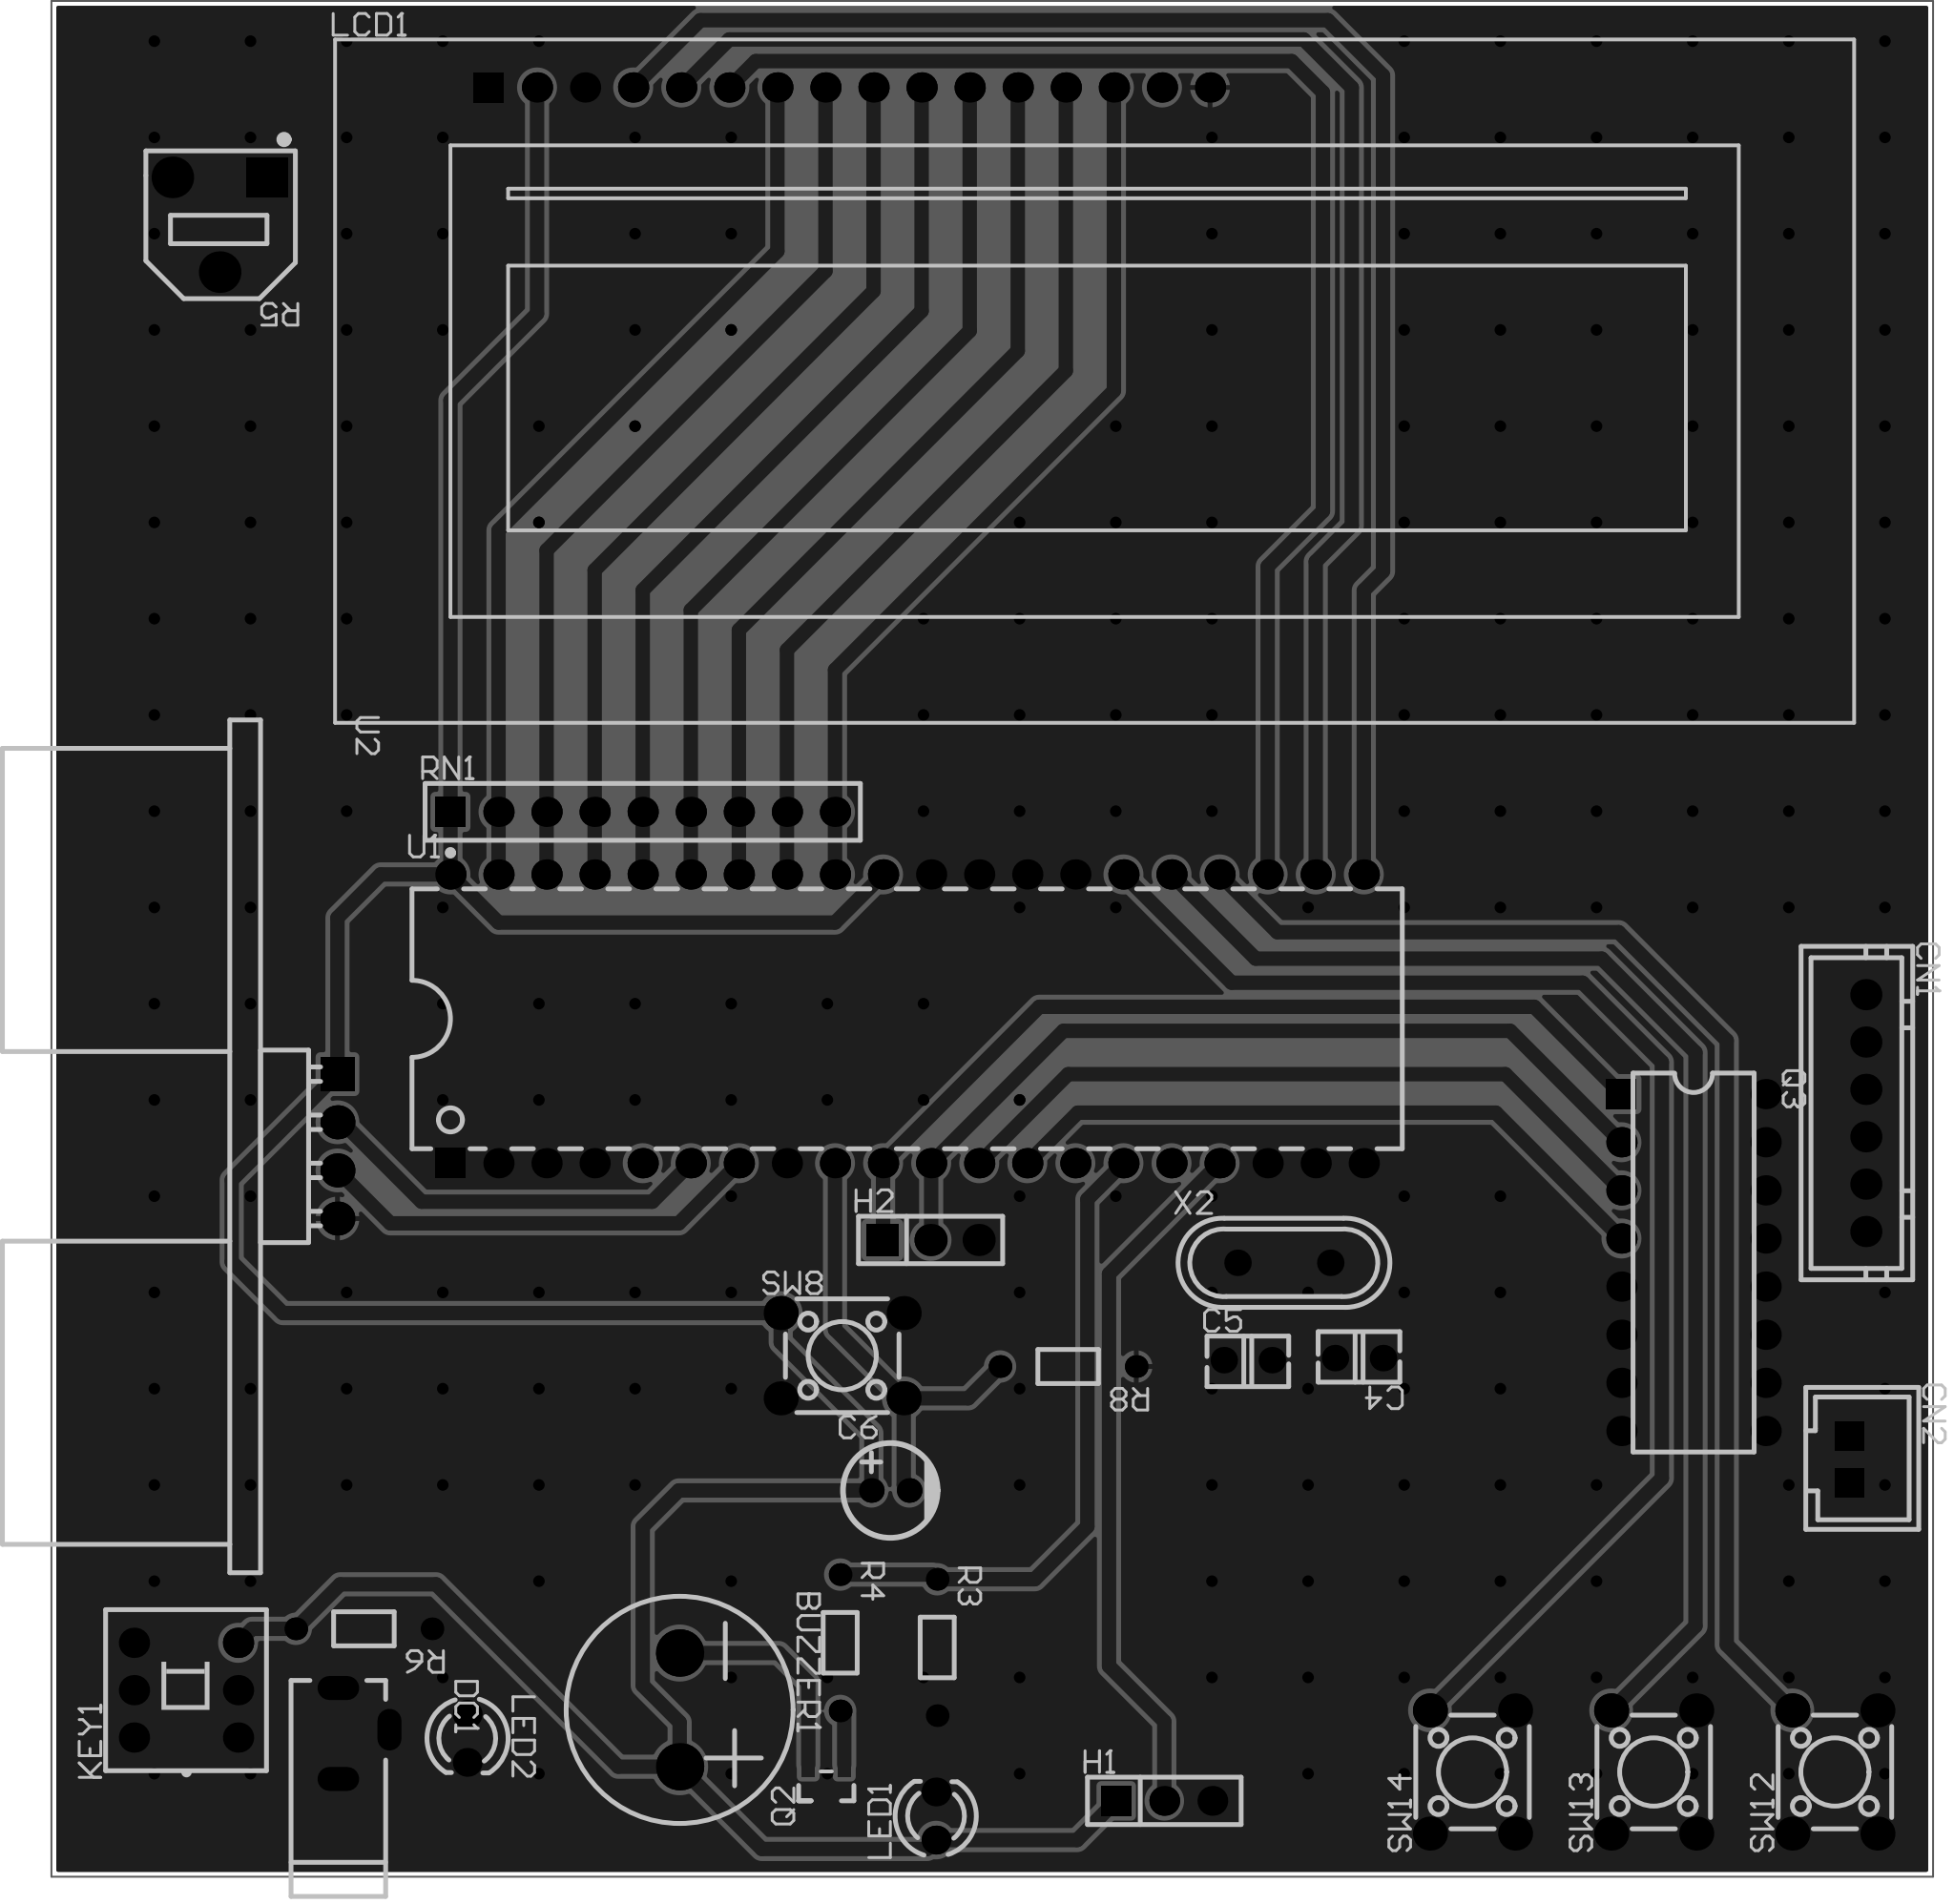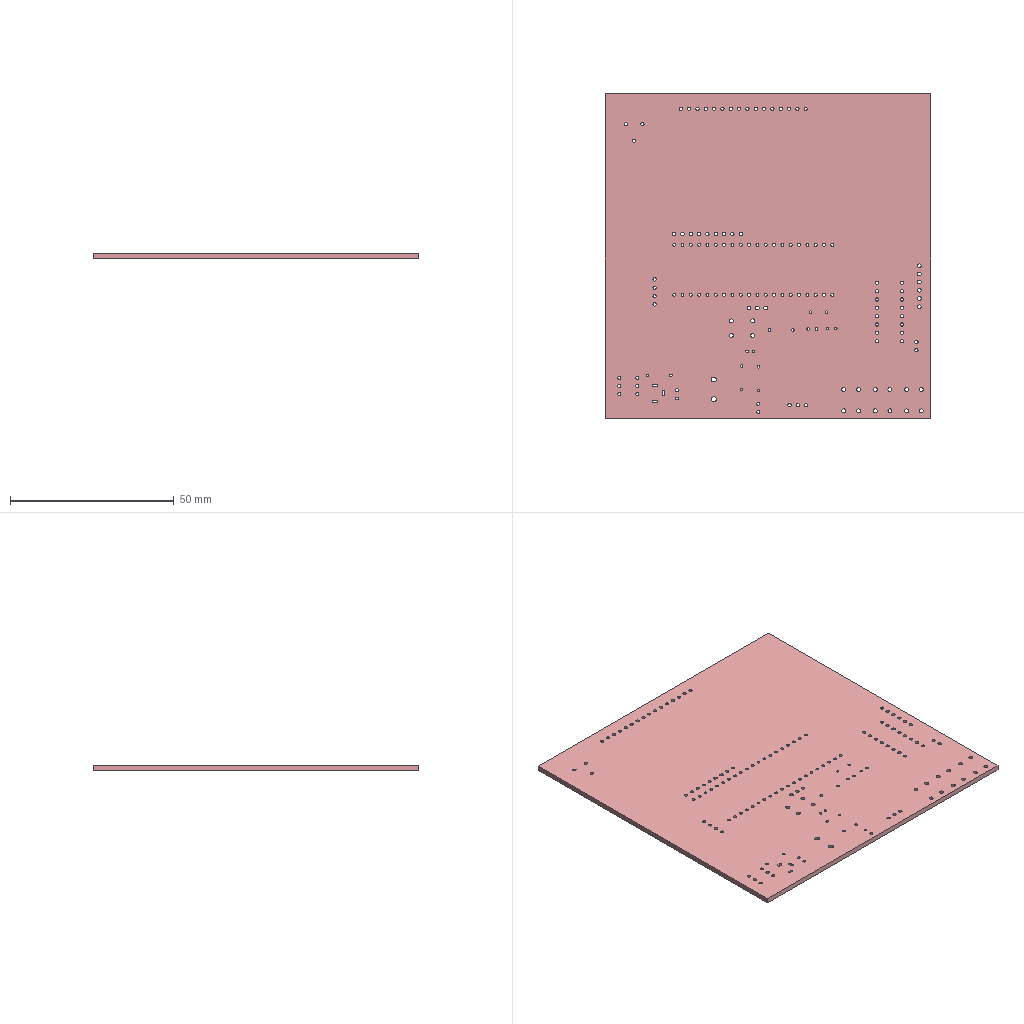Circuit board layout | Altium Designer | box 99.4 x 99 x 1.6 mm
Layer stack:
# Altium Designer layer stack of  (unit mm; dielectric type: 0 none, 1 core, 2 prepreg, 3 surface material)
index,name,kind,layer,copper_thickness_mm,dielectric_type,dielectric_thickness_mm,dielectric_material,dielectric_constant
0,Top Paste Mask Layer,other,,,,,,
1,Top Silkscreen Layer,other,,,,,,
2,Top Solder Mask Layer,dielectric,,,3,0.01,,3.3
3,Top Layer,copper,Top Layer,0.035,,,,
4,Dielectric1,dielectric,,,3,1.51,FR4,4.5
5,Bottom Layer,copper,Bottom Layer,0.035,,,,
6,Bottom Solder Mask Layer,dielectric,,,3,0.01,,3.3
7,Bottom Silkscreen Layer,other,,,,,,
8,Bottom Paste Mask Layer,other,,,,,,
# drill layer pairs: low layer,high layer
drill_pair,Top Layer,Bottom Layer
Part placement:
Designator,Comment,Layer,Footprint,Center-X(mm),Center-Y(mm),Rotation
C4,30pF,TopLayer,CAP-TH_L3.8-W2.5-P2.54-D0.50,166.116,114.046,180
C5,30pF,TopLayer,CAP-TH_L3.8-W2.5-P2.54-D0.50,160.244,113.937,0
C6,10uF,TopLayer,CAP-TH_BD5.0-P2.00-D0.8-FD-10UF50VC110GL,141.351,107.061,0
H2,,TopLayer,HDR-TH_3P-P2.54-V-M,143.48,120.281,0
KEY1,Non-latching switch 8.5×8.5, silent,TopLayer,SW-TH_6P-L8.5-W8.5-P2.54,104.14,96.52,90
LCD1,LCD1602,TopLayer,LCD1602,139.196,181.108,0
LED2,,TopLayer,LED_TH-3mm,118.999,93.98,270
R8,10kΩ,TopLayer,Res_1/8W,150.749,113.602,180
R5,10kΩ,TopLayer,RES-ADJ-SMD_RM065-V1,105.918,173.863,180
R6,1kΩ,TopLayer,Res_1/8W,113.538,99.759,180
SW8,,TopLayer,SW-TH_4P-L6.0-W6.0-P4.50-LS6.5,138.811,114.173,0
SW12,,TopLayer,SW-TH_4P-L6.0-W6.0-P4.50-LS6.5,191.262,92.202,90
SW13,,TopLayer,SW-TH_4P-L6.0-W6.0-P4.50-LS6.5,181.689,92.202,90
SW14,,TopLayer,SW-TH_4P-L6.0-W6.0-P4.50-LS6.5,172.115,92.202,90
U1,STC89C52RC-40I-PDIP40,TopLayer,DIP-40_L52.0-W13.7-P2.54-LS15.2-BL,142.24,131.953,0
X2,11.059MHz,TopLayer,OSC-TH_L11.1-W4.7-P4.88,162.149,119.076,0
DC1,DC-002,TopLayer,DC-IN-TH_DC-3510,113.538,94.234,270
BUZZER1,buzzer,TopLayer,BUZ-TH_BD12.0-P6.00-D0.9-RD,130.22,95.481,270
CN1,XH2.54*6P_through-hole,TopLayer,CONN-TH_XH2.54-6P,192.898,126.978,270
H1,,TopLayer,HDR-TH_3P-P2.54-V-F,155.829,90.678,0
LED1,,TopLayer,LED_TH-3mm,143.766,89.878,90
Q2,,TopLayer,S8550P_SOT,137.967,91.331,90
Q3,ULN2004A,TopLayer,DIP-16_L19.8-W6.5-P2.54-LS7.6-BL,183.794,119.09,270
R3,1KΩ,TopLayer,Res_1/8W,143.829,98.775,270
R4,100Ω,TopLayer,Res_1/8W,138.703,99.022,270
RN1,-,TopLayer,RES-ARRAY-TH_9P-P2.54-D1.0,128.27,142.875,0
U2,HC-SR04,TopLayer,TH_HC-SR04V,112.141,125.222,270
CN2,XH2.54-2PIN-straight pin,TopLayer,CONN-TH_XH2.54-2P,192.009,108.69,270
Pad and via stacks:
# Altium Designer via and pad stacks of  (unit mm). Each distinct definition once, with the count of objects using it.
# via: kind,start_layer,end_layer,hole_mm,diameter_mm,mode(0 simple;1 top-mid-bottom;2 full stack),diameter_per_layer,count,example_net
# pad: kind,layer,hole_mm,hole_type(0 round;1 square;2 slot),plating,top_size,top_shape(1 round;2 rect;3 octagon;9 rounded rect),mid_size,bottom_size,mode,footprint,size_per_layer,count,example
pad,Multi-Layer,0.8,0,plated,1.4x1.4,1,1.4x1.4,1.4x1.4,0,CAP-TH_L3.8-W2.5-P2.54-D0.50,,4,C4.1
pad,Multi-Layer,0.8,0,plated,1.3x1.3,1,1.3x1.3,1.3x1.3,0,CAP-TH_BD5.0-P2.00-D0.8-FD-10UF50VC110GL,,2,C6.2
pad,Multi-Layer,1.1,0,plated,1.7x1.7,2,1.7x1.7,1.7x1.7,0,HDR-TH_3P-P2.54-V-M,,1,H2.1
pad,Multi-Layer,1.1,0,plated,1.7x1.7,1,1.7x1.7,1.7x1.7,0,HDR-TH_3P-P2.54-V-M,,2,H2.2
pad,Multi-Layer,1,0,plated,1.6x1.6,1,1.6x1.6,1.6x1.6,0,SW-TH_6P-L8.5-W8.5-P2.54,,6,KEY1.4
pad,Multi-Layer,1,0,plated,1.6x1.6,1,1.6x1.6,1.6x1.6,0,LCD1602,,15,LCD1.16
pad,Multi-Layer,1,0,plated,1.6x1.6,2,1.6x1.6,1.6x1.6,0,LCD1602,,1,LCD1.1
pad,Multi-Layer,0.9144,0,plated,1.524x1.524,1,1.524x1.524,1.524x1.524,0,LED_TH-3mm,,4,LED2.1
pad,Multi-Layer,0.8001,0,plated,1.199x1.199,1,1.199x1.199,1.199x1.199,0,Res_1/8W,,8,R8.1
pad,Multi-Layer,1,0,plated,2.2x2.1,2,2.2x2.1,2.2x2.1,0,RES-ADJ-SMD_RM065-V1,,1,R5.1
pad,Multi-Layer,1,0,plated,2.2x2.2,1,2.2x2.2,2.2x2.2,0,RES-ADJ-SMD_RM065-V1,,2,R5.3
pad,Multi-Layer,1.2,0,plated,1.8x1.8,1,1.8x1.8,1.8x1.8,0,SW-TH_4P-L6.0-W6.0-P4.50-LS6.5,,16,SW8.1
pad,Multi-Layer,0.889,0,plated,1.6x1.6,1,1.6x1.6,1.6x1.6,0,DIP-40_L52.0-W13.7-P2.54-LS15.2-BL,,39,U1.31
pad,Multi-Layer,0.889,0,plated,1.6x1.6,2,1.6x1.6,1.6x1.6,0,DIP-40_L52.0-W13.7-P2.54-LS15.2-BL,,1,U1.1
pad,Multi-Layer,0.7,0,plated,1.4x1.4,1,1.4x1.4,1.4x1.4,0,OSC-TH_L11.1-W4.7-P4.88,,2,X2.1
pad,Multi-Layer,0.8,2,plated,2.2x1.27,1,2.2x1.27,2.2x1.27,0,DC-IN-TH_DC-3510,,3,DC1.3
pad,Multi-Layer,1.5,0,plated,2.5x2.5,1,2.5x2.5,2.5x2.5,0,BUZ-TH_BD12.0-P6.00-D0.9-RD,,2,BUZZER1.1
pad,Multi-Layer,1.1,0,plated,1.65x1.65,1,1.65x1.65,1.65x1.65,0,CONN-TH_XH2.54-6P,,6,CN1.1
pad,Multi-Layer,1.02,0,plated,1.575x1.575,1,1.575x1.575,1.575x1.575,0,HDR-TH_3P-P2.54-V-F,,2,H1.3
pad,Multi-Layer,1.02,0,plated,1.575x1.575,2,1.575x1.575,1.575x1.575,0,HDR-TH_3P-P2.54-V-F,,1,H1.1
pad,Multi-Layer,1,0,plated,1.6x1.6,1,1.6x1.6,1.6x1.6,0,DIP-16_L19.8-W6.5-P2.54-LS7.6-BL,,15,Q3.16
pad,Multi-Layer,1,0,plated,1.6x1.6,2,1.6x1.6,1.6x1.6,0,DIP-16_L19.8-W6.5-P2.54-LS7.6-BL,,1,Q3.1
pad,Multi-Layer,1,0,plated,1.6x1.6,2,1.6x1.6,1.6x1.6,0,RES-ARRAY-TH_9P-P2.54-D1.0,,1,RN1.1
pad,Multi-Layer,1,0,plated,1.6x1.6,1,1.6x1.6,1.6x1.6,0,RES-ARRAY-TH_9P-P2.54-D1.0,,8,RN1.2
pad,Multi-Layer,1.001,0,plated,1.8x1.8,1,1.8x1.8,1.8x1.8,0,TH_HC-SR04V,,3,U2.4
pad,Multi-Layer,1.001,0,plated,1.8x1.8,2,1.8x1.8,1.8x1.8,0,TH_HC-SR04V,,1,U2.1
pad,Multi-Layer,1,2,plated,1.524x1.524,2,1.524x1.524,1.524x1.524,0,CONN-TH_XH2.54-2P,,2,CN2.1
pad,Top Layer,0,0,plated,0.701x1.25,2,0.701x1.25,0.701x1.25,0,S8550P_SOT,,3,Q2.3
via,Top Layer,Bottom Layer,0.3048,0.61,0,,227,GND
Copper pours:
name,layer,net,type(0 solid;1 hatched;2 none)
Top Layer-GND,Top Layer,GND,0
Bottom Layer-GND,Bottom Layer,GND,0
Design rules, without the lines most boards share:
# Altium Designer design rules of  (exported by Altium Designer, unit mm)
# columns: name | kind | enabled | priority | scope1 | scope2 | descriptor | typed fields (field=value)
creepage | 65 | enabled | 1 | All | All | Creepage Distance Constraint =(0mil) (All),(All) |
copperRegion | 20 | enabled | 1 | (InNet('GND')) | All | Polygon Connect Rule(Relief Connect )(Conductor Width=10mil) (Relief Angle=90 Angle) (Entries=4) (Air Gap Width=10mil) ((InNet('GND'))),(All) | connect_style(0=relief,1=direct,2=none)=0 relief_conductor_width=0.254 relief_entries=4